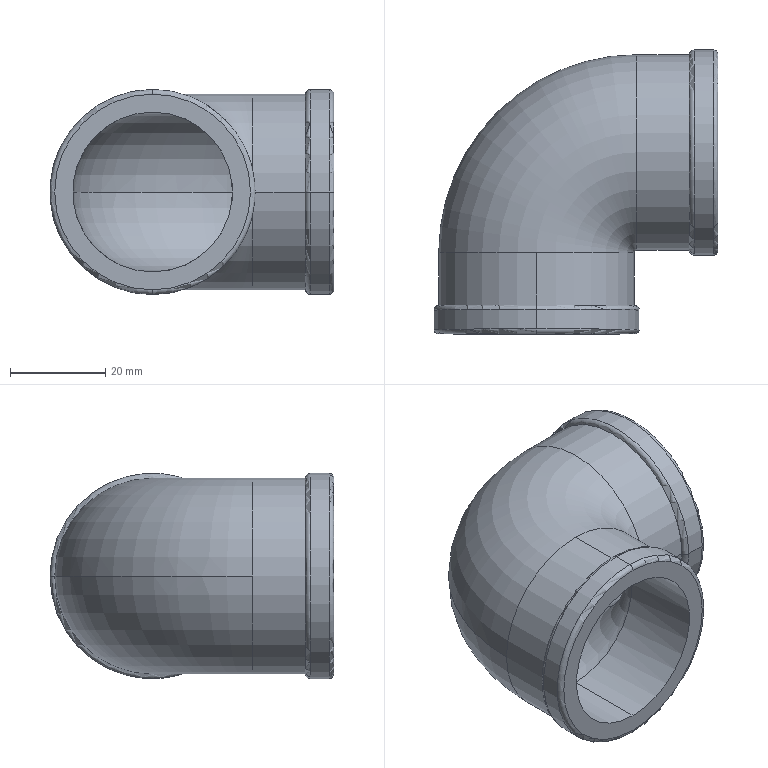Part | SolidWorks | features BossThin 2, Fillet 2, Sweep 1 | 1 solid | 26 faces | box 59.5 x 59.5 x 43 mm | volume 30865 mm3 | torus 12 | cylinder 12 | plane 2 | commonest cylinder face diameters 33.5 x4 41 x4 43 x4
STEP:
#1=CARTESIAN_POINT('',(-16.75,17.,0.));
#2=VERTEX_POINT('',#1);
#3=CARTESIAN_POINT('',(0.,17.,16.75));
#4=VERTEX_POINT('',#3);
#5=CARTESIAN_POINT('',(0.,17.,0.));
#6=DIRECTION('',(0.,1.,0.));
#7=DIRECTION('',(0.,0.,1.));
#8=AXIS2_PLACEMENT_3D('',#5,#6,#7);
#9=CIRCLE('',#8,16.75);
#10=EDGE_CURVE('',#2,#4,#9,.T.);
#11=ORIENTED_EDGE('',*,*,#10,.F.);
#12=CARTESIAN_POINT('',(21.,54.75,0.));
#13=VERTEX_POINT('',#12);
#14=CARTESIAN_POINT('',(21.,17.,0.));
#15=DIRECTION('',(0.,0.,-1.));
#16=DIRECTION('',(-1.,0.,0.));
#17=AXIS2_PLACEMENT_3D('',#14,#15,#16);
#18=CIRCLE('',#17,37.75);
#19=EDGE_CURVE('',#2,#13,#18,.T.);
#20=ORIENTED_EDGE('',*,*,#19,.T.);
#21=CARTESIAN_POINT('',(21.,21.25,0.));
#22=VERTEX_POINT('',#21);
#23=CARTESIAN_POINT('',(21.,38.,0.));
#24=DIRECTION('',(1.,0.,0.));
#25=DIRECTION('',(0.,0.,1.));
#26=AXIS2_PLACEMENT_3D('',#23,#24,#25);
#27=CIRCLE('',#26,16.75);
#28=EDGE_CURVE('',#13,#22,#27,.T.);
#29=ORIENTED_EDGE('',*,*,#28,.T.);
#30=CARTESIAN_POINT('',(16.75,17.,0.));
#31=VERTEX_POINT('',#30);
#32=CARTESIAN_POINT('',(21.,17.,0.));
#33=DIRECTION('',(0.,0.,-1.));
#34=DIRECTION('',(-1.,0.,0.));
#35=AXIS2_PLACEMENT_3D('',#32,#33,#34);
#36=CIRCLE('',#35,4.25);
#37=EDGE_CURVE('',#31,#22,#36,.T.);
#38=ORIENTED_EDGE('',*,*,#37,.F.);
#39=CARTESIAN_POINT('',(0.,17.,0.));
#40=DIRECTION('',(0.,1.,0.));
#41=DIRECTION('',(0.,0.,1.));
#42=AXIS2_PLACEMENT_3D('',#39,#40,#41);
#43=CIRCLE('',#42,16.75);
#44=EDGE_CURVE('',#4,#31,#43,.T.);
#45=ORIENTED_EDGE('',*,*,#44,.F.);
#46=EDGE_LOOP('',(#11,#20,#29,#38,#45));
#47=FACE_OUTER_BOUND('',#46,.T.);
#48=CARTESIAN_POINT('',(21.,17.,0.));
#49=DIRECTION('',(0.,0.,-1.));
#50=DIRECTION('',(-1.,0.,0.));
#51=AXIS2_PLACEMENT_3D('',#48,#49,#50);
#52=TOROIDAL_SURFACE('',#51,21.,16.75);
#53=ADVANCED_FACE('',(#47),#52,.F.);
#54=CARTESIAN_POINT('',(0.,17.,-20.5));
#55=VERTEX_POINT('',#54);
#56=CARTESIAN_POINT('',(-20.5,17.,0.));
#57=VERTEX_POINT('',#56);
#58=CARTESIAN_POINT('',(0.,17.,0.));
#59=DIRECTION('',(0.,1.,0.));
#60=DIRECTION('',(0.,0.,1.));
#61=AXIS2_PLACEMENT_3D('',#58,#59,#60);
#62=CIRCLE('',#61,20.5);
#63=EDGE_CURVE('',#55,#57,#62,.T.);
#64=ORIENTED_EDGE('',*,*,#63,.T.);
#65=CARTESIAN_POINT('',(21.,58.5,0.));
#66=VERTEX_POINT('',#65);
#67=CARTESIAN_POINT('',(21.,17.,0.));
#68=DIRECTION('',(0.,0.,-1.));
#69=DIRECTION('',(-1.,0.,0.));
#70=AXIS2_PLACEMENT_3D('',#67,#68,#69);
#71=CIRCLE('',#70,41.5);
#72=EDGE_CURVE('',#57,#66,#71,.T.);
#73=ORIENTED_EDGE('',*,*,#72,.T.);
#74=CARTESIAN_POINT('',(21.,17.5,0.));
#75=VERTEX_POINT('',#74);
#76=CARTESIAN_POINT('',(21.,38.,0.));
#77=DIRECTION('',(1.,0.,0.));
#78=DIRECTION('',(0.,0.,1.));
#79=AXIS2_PLACEMENT_3D('',#76,#77,#78);
#80=CIRCLE('',#79,20.5);
#81=EDGE_CURVE('',#75,#66,#80,.T.);
#82=ORIENTED_EDGE('',*,*,#81,.F.);
#83=CARTESIAN_POINT('',(20.5,17.,0.));
#84=VERTEX_POINT('',#83);
#85=CARTESIAN_POINT('',(21.,17.,0.));
#86=DIRECTION('',(0.,0.,-1.));
#87=DIRECTION('',(-1.,0.,0.));
#88=AXIS2_PLACEMENT_3D('',#85,#86,#87);
#89=CIRCLE('',#88,0.5);
#90=EDGE_CURVE('',#84,#75,#89,.T.);
#91=ORIENTED_EDGE('',*,*,#90,.F.);
#92=CARTESIAN_POINT('',(0.,17.,0.));
#93=DIRECTION('',(0.,1.,0.));
#94=DIRECTION('',(0.,0.,1.));
#95=AXIS2_PLACEMENT_3D('',#92,#93,#94);
#96=CIRCLE('',#95,20.5);
#97=EDGE_CURVE('',#84,#55,#96,.T.);
#98=ORIENTED_EDGE('',*,*,#97,.T.);
#99=EDGE_LOOP('',(#64,#73,#82,#91,#98));
#100=FACE_OUTER_BOUND('',#99,.T.);
#101=CARTESIAN_POINT('',(21.,17.,0.));
#102=DIRECTION('',(0.,0.,-1.));
#103=DIRECTION('',(-1.,0.,0.));
#104=AXIS2_PLACEMENT_3D('',#101,#102,#103);
#105=TOROIDAL_SURFACE('',#104,21.,20.5);
#106=ADVANCED_FACE('',(#100),#105,.T.);
#107=CARTESIAN_POINT('',(37.,16.5,0.));
#108=VERTEX_POINT('',#107);
#109=CARTESIAN_POINT('',(37.,59.5,0.));
#110=VERTEX_POINT('',#109);
#111=CARTESIAN_POINT('',(37.,38.,0.));
#112=DIRECTION('',(-1.,0.,0.));
#113=DIRECTION('',(0.,1.,0.));
#114=AXIS2_PLACEMENT_3D('',#111,#112,#113);
#115=CIRCLE('',#114,21.5);
#116=EDGE_CURVE('',#108,#110,#115,.T.);
#117=ORIENTED_EDGE('',*,*,#116,.F.);
#118=CARTESIAN_POINT('',(38.,17.5,0.));
#119=VERTEX_POINT('',#118);
#120=CARTESIAN_POINT('',(37.,17.5,0.));
#121=DIRECTION('',(0.,0.,1.));
#122=DIRECTION('',(0.,-1.,0.));
#123=AXIS2_PLACEMENT_3D('',#120,#121,#122);
#124=CIRCLE('',#123,1.);
#125=EDGE_CURVE('',#108,#119,#124,.T.);
#126=ORIENTED_EDGE('',*,*,#125,.T.);
#127=CARTESIAN_POINT('',(38.,58.5,0.));
#128=VERTEX_POINT('',#127);
#129=CARTESIAN_POINT('',(38.,38.,0.));
#130=DIRECTION('',(1.,0.,0.));
#131=DIRECTION('',(0.,1.,0.));
#132=AXIS2_PLACEMENT_3D('',#129,#130,#131);
#133=CIRCLE('',#132,20.5);
#134=EDGE_CURVE('',#128,#119,#133,.T.);
#135=ORIENTED_EDGE('',*,*,#134,.F.);
#136=CARTESIAN_POINT('',(37.,58.5,0.));
#137=DIRECTION('',(0.,0.,-1.));
#138=DIRECTION('',(-1.,0.,0.));
#139=AXIS2_PLACEMENT_3D('',#136,#137,#138);
#140=CIRCLE('',#139,1.);
#141=EDGE_CURVE('',#110,#128,#140,.T.);
#142=ORIENTED_EDGE('',*,*,#141,.F.);
#143=EDGE_LOOP('',(#117,#126,#135,#142));
#144=FACE_OUTER_BOUND('',#143,.T.);
#145=CARTESIAN_POINT('',(37.,38.,0.));
#146=DIRECTION('',(1.,0.,0.));
#147=DIRECTION('',(0.,1.,0.));
#148=AXIS2_PLACEMENT_3D('',#145,#146,#147);
#149=TOROIDAL_SURFACE('',#148,20.5,1.);
#150=ADVANCED_FACE('',(#144),#149,.T.);
#151=CARTESIAN_POINT('',(32.,58.5,0.));
#152=VERTEX_POINT('',#151);
#153=CARTESIAN_POINT('',(32.,17.5,0.));
#154=VERTEX_POINT('',#153);
#155=CARTESIAN_POINT('',(32.,38.,0.));
#156=DIRECTION('',(1.,0.,0.));
#157=DIRECTION('',(0.,1.,0.));
#158=AXIS2_PLACEMENT_3D('',#155,#156,#157);
#159=CIRCLE('',#158,20.5);
#160=EDGE_CURVE('',#152,#154,#159,.T.);
#161=ORIENTED_EDGE('',*,*,#160,.T.);
#162=CARTESIAN_POINT('',(33.,16.5,0.));
#163=VERTEX_POINT('',#162);
#164=CARTESIAN_POINT('',(33.,17.5,0.));
#165=DIRECTION('',(0.,0.,1.));
#166=DIRECTION('',(0.,-1.,0.));
#167=AXIS2_PLACEMENT_3D('',#164,#165,#166);
#168=CIRCLE('',#167,1.);
#169=EDGE_CURVE('',#154,#163,#168,.T.);
#170=ORIENTED_EDGE('',*,*,#169,.T.);
#171=CARTESIAN_POINT('',(33.,59.5,0.));
#172=VERTEX_POINT('',#171);
#173=CARTESIAN_POINT('',(33.,38.,0.));
#174=DIRECTION('',(1.,0.,0.));
#175=DIRECTION('',(0.,1.,0.));
#176=AXIS2_PLACEMENT_3D('',#173,#174,#175);
#177=CIRCLE('',#176,21.5);
#178=EDGE_CURVE('',#172,#163,#177,.T.);
#179=ORIENTED_EDGE('',*,*,#178,.F.);
#180=CARTESIAN_POINT('',(33.,58.5,0.));
#181=DIRECTION('',(0.,0.,-1.));
#182=DIRECTION('',(-1.,0.,0.));
#183=AXIS2_PLACEMENT_3D('',#180,#181,#182);
#184=CIRCLE('',#183,1.);
#185=EDGE_CURVE('',#152,#172,#184,.T.);
#186=ORIENTED_EDGE('',*,*,#185,.F.);
#187=EDGE_LOOP('',(#161,#170,#179,#186));
#188=FACE_OUTER_BOUND('',#187,.T.);
#189=CARTESIAN_POINT('',(33.,38.,0.));
#190=DIRECTION('',(1.,0.,0.));
#191=DIRECTION('',(0.,1.,0.));
#192=AXIS2_PLACEMENT_3D('',#189,#190,#191);
#193=TOROIDAL_SURFACE('',#192,20.5,1.);
#194=ADVANCED_FACE('',(#188),#193,.T.);
#195=ORIENTED_EDGE('',*,*,#178,.T.);
#196=CARTESIAN_POINT('',(32.,16.5,0.));
#197=DIRECTION('',(1.,0.,0.));
#198=VECTOR('',#197,1000.);
#199=LINE('',#196,#198);
#200=EDGE_CURVE('',#163,#108,#199,.T.);
#201=ORIENTED_EDGE('',*,*,#200,.T.);
#202=ORIENTED_EDGE('',*,*,#116,.T.);
#203=CARTESIAN_POINT('',(32.,59.5,0.));
#204=DIRECTION('',(1.,0.,0.));
#205=VECTOR('',#204,1000.);
#206=LINE('',#203,#205);
#207=EDGE_CURVE('',#172,#110,#206,.T.);
#208=ORIENTED_EDGE('',*,*,#207,.F.);
#209=EDGE_LOOP('',(#195,#201,#202,#208));
#210=FACE_OUTER_BOUND('',#209,.T.);
#211=CARTESIAN_POINT('',(32.,38.,0.));
#212=DIRECTION('',(1.,0.,0.));
#213=DIRECTION('',(0.,1.,0.));
#214=AXIS2_PLACEMENT_3D('',#211,#212,#213);
#215=CYLINDRICAL_SURFACE('',#214,21.5);
#216=ADVANCED_FACE('',(#210),#215,.T.);
#217=CARTESIAN_POINT('',(0.,0.,-20.5));
#218=VERTEX_POINT('',#217);
#219=CARTESIAN_POINT('',(0.,0.,20.5));
#220=VERTEX_POINT('',#219);
#221=CARTESIAN_POINT('',(0.,0.,0.));
#222=DIRECTION('',(0.,-1.,0.));
#223=DIRECTION('',(0.,0.,1.));
#224=AXIS2_PLACEMENT_3D('',#221,#222,#223);
#225=CIRCLE('',#224,20.5);
#226=EDGE_CURVE('',#218,#220,#225,.T.);
#227=ORIENTED_EDGE('',*,*,#226,.F.);
#228=CARTESIAN_POINT('',(0.,1.,-21.5));
#229=VERTEX_POINT('',#228);
#230=CARTESIAN_POINT('',(0.,1.,-20.5));
#231=DIRECTION('',(1.,0.,0.));
#232=DIRECTION('',(0.,0.,-1.));
#233=AXIS2_PLACEMENT_3D('',#230,#231,#232);
#234=CIRCLE('',#233,1.);
#235=EDGE_CURVE('',#218,#229,#234,.T.);
#236=ORIENTED_EDGE('',*,*,#235,.T.);
#237=CARTESIAN_POINT('',(0.,1.,21.5));
#238=VERTEX_POINT('',#237);
#239=CARTESIAN_POINT('',(0.,1.,0.));
#240=DIRECTION('',(0.,1.,0.));
#241=DIRECTION('',(0.,0.,1.));
#242=AXIS2_PLACEMENT_3D('',#239,#240,#241);
#243=CIRCLE('',#242,21.5);
#244=EDGE_CURVE('',#238,#229,#243,.T.);
#245=ORIENTED_EDGE('',*,*,#244,.F.);
#246=CARTESIAN_POINT('',(0.,1.,20.5));
#247=DIRECTION('',(-1.,0.,0.));
#248=DIRECTION('',(0.,0.,1.));
#249=AXIS2_PLACEMENT_3D('',#246,#247,#248);
#250=CIRCLE('',#249,1.);
#251=EDGE_CURVE('',#220,#238,#250,.T.);
#252=ORIENTED_EDGE('',*,*,#251,.F.);
#253=EDGE_LOOP('',(#227,#236,#245,#252));
#254=FACE_OUTER_BOUND('',#253,.T.);
#255=CARTESIAN_POINT('',(0.,1.,0.));
#256=DIRECTION('',(0.,1.,0.));
#257=DIRECTION('',(0.,0.,1.));
#258=AXIS2_PLACEMENT_3D('',#255,#256,#257);
#259=TOROIDAL_SURFACE('',#258,20.5,1.);
#260=ADVANCED_FACE('',(#254),#259,.T.);
#261=CARTESIAN_POINT('',(0.,6.,-20.5));
#262=VERTEX_POINT('',#261);
#263=CARTESIAN_POINT('',(0.,6.,20.5));
#264=VERTEX_POINT('',#263);
#265=CARTESIAN_POINT('',(0.,6.,0.));
#266=DIRECTION('',(0.,-1.,0.));
#267=DIRECTION('',(0.,0.,-1.));
#268=AXIS2_PLACEMENT_3D('',#265,#266,#267);
#269=CIRCLE('',#268,20.5);
#270=EDGE_CURVE('',#262,#264,#269,.T.);
#271=ORIENTED_EDGE('',*,*,#270,.T.);
#272=CARTESIAN_POINT('',(0.,5.,21.5));
#273=VERTEX_POINT('',#272);
#274=CARTESIAN_POINT('',(0.,5.,20.5));
#275=DIRECTION('',(1.,0.,0.));
#276=DIRECTION('',(0.,0.,-1.));
#277=AXIS2_PLACEMENT_3D('',#274,#275,#276);
#278=CIRCLE('',#277,1.);
#279=EDGE_CURVE('',#264,#273,#278,.T.);
#280=ORIENTED_EDGE('',*,*,#279,.T.);
#281=CARTESIAN_POINT('',(0.,5.,-21.5));
#282=VERTEX_POINT('',#281);
#283=CARTESIAN_POINT('',(0.,5.,0.));
#284=DIRECTION('',(0.,-1.,0.));
#285=DIRECTION('',(0.,0.,-1.));
#286=AXIS2_PLACEMENT_3D('',#283,#284,#285);
#287=CIRCLE('',#286,21.5);
#288=EDGE_CURVE('',#282,#273,#287,.T.);
#289=ORIENTED_EDGE('',*,*,#288,.F.);
#290=CARTESIAN_POINT('',(0.,5.,-20.5));
#291=DIRECTION('',(-1.,0.,0.));
#292=DIRECTION('',(0.,0.,1.));
#293=AXIS2_PLACEMENT_3D('',#290,#291,#292);
#294=CIRCLE('',#293,1.);
#295=EDGE_CURVE('',#262,#282,#294,.T.);
#296=ORIENTED_EDGE('',*,*,#295,.F.);
#297=EDGE_LOOP('',(#271,#280,#289,#296));
#298=FACE_OUTER_BOUND('',#297,.T.);
#299=CARTESIAN_POINT('',(0.,5.,0.));
#300=DIRECTION('',(0.,-1.,0.));
#301=DIRECTION('',(0.,0.,-1.));
#302=AXIS2_PLACEMENT_3D('',#299,#300,#301);
#303=TOROIDAL_SURFACE('',#302,20.5,1.);
#304=ADVANCED_FACE('',(#298),#303,.T.);
#305=ORIENTED_EDGE('',*,*,#288,.T.);
#306=CARTESIAN_POINT('',(0.,6.,21.5));
#307=DIRECTION('',(0.,-1.,0.));
#308=VECTOR('',#307,1000.);
#309=LINE('',#306,#308);
#310=EDGE_CURVE('',#273,#238,#309,.T.);
#311=ORIENTED_EDGE('',*,*,#310,.T.);
#312=ORIENTED_EDGE('',*,*,#244,.T.);
#313=CARTESIAN_POINT('',(0.,6.,-21.5));
#314=DIRECTION('',(0.,-1.,0.));
#315=VECTOR('',#314,1000.);
#316=LINE('',#313,#315);
#317=EDGE_CURVE('',#282,#229,#316,.T.);
#318=ORIENTED_EDGE('',*,*,#317,.F.);
#319=EDGE_LOOP('',(#305,#311,#312,#318));
#320=FACE_OUTER_BOUND('',#319,.T.);
#321=CARTESIAN_POINT('',(0.,6.,0.));
#322=DIRECTION('',(0.,-1.,0.));
#323=DIRECTION('',(0.,0.,-1.));
#324=AXIS2_PLACEMENT_3D('',#321,#322,#323);
#325=CYLINDRICAL_SURFACE('',#324,21.5);
#326=ADVANCED_FACE('',(#320),#325,.T.);
#327=CARTESIAN_POINT('',(0.,17.,-16.75));
#328=VERTEX_POINT('',#327);
#329=CARTESIAN_POINT('',(0.,17.,0.));
#330=DIRECTION('',(0.,1.,0.));
#331=DIRECTION('',(0.,0.,1.));
#332=AXIS2_PLACEMENT_3D('',#329,#330,#331);
#333=CIRCLE('',#332,16.75);
#334=EDGE_CURVE('',#328,#2,#333,.T.);
#335=ORIENTED_EDGE('',*,*,#334,.T.);
#336=ORIENTED_EDGE('',*,*,#10,.T.);
#337=CARTESIAN_POINT('',(0.,0.,16.75));
#338=VERTEX_POINT('',#337);
#339=CARTESIAN_POINT('',(0.,17.,16.75));
#340=DIRECTION('',(0.,-1.,0.));
#341=VECTOR('',#340,1000.);
#342=LINE('',#339,#341);
#343=EDGE_CURVE('',#4,#338,#342,.T.);
#344=ORIENTED_EDGE('',*,*,#343,.T.);
#345=CARTESIAN_POINT('',(0.,0.,-16.75));
#346=VERTEX_POINT('',#345);
#347=CARTESIAN_POINT('',(0.,0.,0.));
#348=DIRECTION('',(0.,1.,0.));
#349=DIRECTION('',(0.,0.,1.));
#350=AXIS2_PLACEMENT_3D('',#347,#348,#349);
#351=CIRCLE('',#350,16.75);
#352=EDGE_CURVE('',#346,#338,#351,.T.);
#353=ORIENTED_EDGE('',*,*,#352,.F.);
#354=CARTESIAN_POINT('',(0.,17.,-16.75));
#355=DIRECTION('',(0.,-1.,0.));
#356=VECTOR('',#355,1000.);
#357=LINE('',#354,#356);
#358=EDGE_CURVE('',#328,#346,#357,.T.);
#359=ORIENTED_EDGE('',*,*,#358,.F.);
#360=EDGE_LOOP('',(#335,#336,#344,#353,#359));
#361=FACE_OUTER_BOUND('',#360,.T.);
#362=CARTESIAN_POINT('',(0.,17.,0.));
#363=DIRECTION('',(0.,-1.,0.));
#364=DIRECTION('',(0.,0.,-1.));
#365=AXIS2_PLACEMENT_3D('',#362,#363,#364);
#366=CYLINDRICAL_SURFACE('',#365,16.75);
#367=ADVANCED_FACE('',(#361),#366,.F.);
#368=CARTESIAN_POINT('',(21.,38.,0.));
#369=DIRECTION('',(1.,0.,0.));
#370=DIRECTION('',(0.,0.,1.));
#371=AXIS2_PLACEMENT_3D('',#368,#369,#370);
#372=CIRCLE('',#371,16.75);
#373=EDGE_CURVE('',#22,#13,#372,.T.);
#374=ORIENTED_EDGE('',*,*,#373,.F.);
#375=CARTESIAN_POINT('',(38.,21.25,0.));
#376=VERTEX_POINT('',#375);
#377=CARTESIAN_POINT('',(21.,21.25,0.));
#378=DIRECTION('',(1.,0.,0.));
#379=VECTOR('',#378,1000.);
#380=LINE('',#377,#379);
#381=EDGE_CURVE('',#22,#376,#380,.T.);
#382=ORIENTED_EDGE('',*,*,#381,.T.);
#383=CARTESIAN_POINT('',(38.,54.75,0.));
#384=VERTEX_POINT('',#383);
#385=CARTESIAN_POINT('',(38.,38.,0.));
#386=DIRECTION('',(1.,0.,0.));
#387=DIRECTION('',(0.,0.,1.));
#388=AXIS2_PLACEMENT_3D('',#385,#386,#387);
#389=CIRCLE('',#388,16.75);
#390=EDGE_CURVE('',#376,#384,#389,.T.);
#391=ORIENTED_EDGE('',*,*,#390,.T.);
#392=CARTESIAN_POINT('',(21.,54.75,0.));
#393=DIRECTION('',(1.,0.,0.));
#394=VECTOR('',#393,1000.);
#395=LINE('',#392,#394);
#396=EDGE_CURVE('',#13,#384,#395,.T.);
#397=ORIENTED_EDGE('',*,*,#396,.F.);
#398=EDGE_LOOP('',(#374,#382,#391,#397));
#399=FACE_OUTER_BOUND('',#398,.T.);
#400=CARTESIAN_POINT('',(21.,38.,0.));
#401=DIRECTION('',(1.,0.,0.));
#402=DIRECTION('',(0.,1.,0.));
#403=AXIS2_PLACEMENT_3D('',#400,#401,#402);
#404=CYLINDRICAL_SURFACE('',#403,16.75);
#405=ADVANCED_FACE('',(#399),#404,.F.);
#406=CARTESIAN_POINT('',(0.,17.,20.5));
#407=VERTEX_POINT('',#406);
#408=CARTESIAN_POINT('',(0.,17.,0.));
#409=DIRECTION('',(0.,1.,0.));
#410=DIRECTION('',(0.,0.,1.));
#411=AXIS2_PLACEMENT_3D('',#408,#409,#410);
#412=CIRCLE('',#411,20.5);
#413=EDGE_CURVE('',#407,#84,#412,.T.);
#414=ORIENTED_EDGE('',*,*,#413,.F.);
#415=CARTESIAN_POINT('',(0.,17.,20.5));
#416=DIRECTION('',(0.,-1.,0.));
#417=VECTOR('',#416,1000.);
#418=LINE('',#415,#417);
#419=EDGE_CURVE('',#407,#264,#418,.T.);
#420=ORIENTED_EDGE('',*,*,#419,.T.);
#421=ORIENTED_EDGE('',*,*,#270,.F.);
#422=CARTESIAN_POINT('',(0.,17.,-20.5));
#423=DIRECTION('',(0.,-1.,0.));
#424=VECTOR('',#423,1000.);
#425=LINE('',#422,#424);
#426=EDGE_CURVE('',#55,#262,#425,.T.);
#427=ORIENTED_EDGE('',*,*,#426,.F.);
#428=ORIENTED_EDGE('',*,*,#97,.F.);
#429=EDGE_LOOP('',(#414,#420,#421,#427,#428));
#430=FACE_OUTER_BOUND('',#429,.T.);
#431=CARTESIAN_POINT('',(0.,17.,0.));
#432=DIRECTION('',(0.,-1.,0.));
#433=DIRECTION('',(0.,0.,-1.));
#434=AXIS2_PLACEMENT_3D('',#431,#432,#433);
#435=CYLINDRICAL_SURFACE('',#434,20.5);
#436=ADVANCED_FACE('',(#430),#435,.T.);
#437=CARTESIAN_POINT('',(21.,38.,0.));
#438=DIRECTION('',(1.,0.,0.));
#439=DIRECTION('',(0.,0.,1.));
#440=AXIS2_PLACEMENT_3D('',#437,#438,#439);
#441=CIRCLE('',#440,20.5);
#442=EDGE_CURVE('',#66,#75,#441,.T.);
#443=ORIENTED_EDGE('',*,*,#442,.T.);
#444=CARTESIAN_POINT('',(21.,17.5,0.));
#445=DIRECTION('',(1.,0.,0.));
#446=VECTOR('',#445,1000.);
#447=LINE('',#444,#446);
#448=EDGE_CURVE('',#75,#154,#447,.T.);
#449=ORIENTED_EDGE('',*,*,#448,.T.);
#450=ORIENTED_EDGE('',*,*,#160,.F.);
#451=CARTESIAN_POINT('',(21.,58.5,0.));
#452=DIRECTION('',(1.,0.,0.));
#453=VECTOR('',#452,1000.);
#454=LINE('',#451,#453);
#455=EDGE_CURVE('',#66,#152,#454,.T.);
#456=ORIENTED_EDGE('',*,*,#455,.F.);
#457=EDGE_LOOP('',(#443,#449,#450,#456));
#458=FACE_OUTER_BOUND('',#457,.T.);
#459=CARTESIAN_POINT('',(21.,38.,0.));
#460=DIRECTION('',(1.,0.,0.));
#461=DIRECTION('',(0.,1.,0.));
#462=AXIS2_PLACEMENT_3D('',#459,#460,#461);
#463=CYLINDRICAL_SURFACE('',#462,20.5);
#464=ADVANCED_FACE('',(#458),#463,.T.);
#465=ORIENTED_EDGE('',*,*,#448,.F.);
#466=ORIENTED_EDGE('',*,*,#81,.T.);
#467=ORIENTED_EDGE('',*,*,#455,.T.);
#468=CARTESIAN_POINT('',(32.,38.,0.));
#469=DIRECTION('',(1.,0.,0.));
#470=DIRECTION('',(0.,1.,0.));
#471=AXIS2_PLACEMENT_3D('',#468,#469,#470);
#472=CIRCLE('',#471,20.5);
#473=EDGE_CURVE('',#154,#152,#472,.T.);
#474=ORIENTED_EDGE('',*,*,#473,.F.);
#475=EDGE_LOOP('',(#465,#466,#467,#474));
#476=FACE_OUTER_BOUND('',#475,.T.);
#477=CARTESIAN_POINT('',(21.,38.,0.));
#478=DIRECTION('',(1.,0.,0.));
#479=DIRECTION('',(0.,1.,0.));
#480=AXIS2_PLACEMENT_3D('',#477,#478,#479);
#481=CYLINDRICAL_SURFACE('',#480,20.5);
#482=ADVANCED_FACE('',(#476),#481,.T.);
#483=ORIENTED_EDGE('',*,*,#419,.F.);
#484=CARTESIAN_POINT('',(0.,17.,0.));
#485=DIRECTION('',(0.,1.,0.));
#486=DIRECTION('',(0.,0.,1.));
#487=AXIS2_PLACEMENT_3D('',#484,#485,#486);
#488=CIRCLE('',#487,20.5);
#489=EDGE_CURVE('',#57,#407,#488,.T.);
#490=ORIENTED_EDGE('',*,*,#489,.F.);
#491=ORIENTED_EDGE('',*,*,#63,.F.);
#492=ORIENTED_EDGE('',*,*,#426,.T.);
#493=CARTESIAN_POINT('',(0.,6.,0.));
#494=DIRECTION('',(0.,-1.,0.));
#495=DIRECTION('',(0.,0.,-1.));
#496=AXIS2_PLACEMENT_3D('',#493,#494,#495);
#497=CIRCLE('',#496,20.5);
#498=EDGE_CURVE('',#264,#262,#497,.T.);
#499=ORIENTED_EDGE('',*,*,#498,.F.);
#500=EDGE_LOOP('',(#483,#490,#491,#492,#499));
#501=FACE_OUTER_BOUND('',#500,.T.);
#502=CARTESIAN_POINT('',(0.,17.,0.));
#503=DIRECTION('',(0.,-1.,0.));
#504=DIRECTION('',(0.,0.,-1.));
#505=AXIS2_PLACEMENT_3D('',#502,#503,#504);
#506=CYLINDRICAL_SURFACE('',#505,20.5);
#507=ADVANCED_FACE('',(#501),#506,.T.);
#508=ORIENTED_EDGE('',*,*,#381,.F.);
#509=ORIENTED_EDGE('',*,*,#28,.F.);
#510=ORIENTED_EDGE('',*,*,#396,.T.);
#511=CARTESIAN_POINT('',(38.,38.,0.));
#512=DIRECTION('',(1.,0.,0.));
#513=DIRECTION('',(0.,0.,1.));
#514=AXIS2_PLACEMENT_3D('',#511,#512,#513);
#515=CIRCLE('',#514,16.75);
#516=EDGE_CURVE('',#384,#376,#515,.T.);
#517=ORIENTED_EDGE('',*,*,#516,.T.);
#518=EDGE_LOOP('',(#508,#509,#510,#517));
#519=FACE_OUTER_BOUND('',#518,.T.);
#520=CARTESIAN_POINT('',(21.,38.,0.));
#521=DIRECTION('',(1.,0.,0.));
#522=DIRECTION('',(0.,1.,0.));
#523=AXIS2_PLACEMENT_3D('',#520,#521,#522);
#524=CYLINDRICAL_SURFACE('',#523,16.75);
#525=ADVANCED_FACE('',(#519),#524,.F.);
#526=ORIENTED_EDGE('',*,*,#72,.F.);
#527=ORIENTED_EDGE('',*,*,#489,.T.);
#528=ORIENTED_EDGE('',*,*,#413,.T.);
#529=ORIENTED_EDGE('',*,*,#90,.T.);
#530=ORIENTED_EDGE('',*,*,#442,.F.);
#531=EDGE_LOOP('',(#526,#527,#528,#529,#530));
#532=FACE_OUTER_BOUND('',#531,.T.);
#533=CARTESIAN_POINT('',(21.,17.,0.));
#534=DIRECTION('',(0.,0.,-1.));
#535=DIRECTION('',(-1.,0.,0.));
#536=AXIS2_PLACEMENT_3D('',#533,#534,#535);
#537=TOROIDAL_SURFACE('',#536,21.,20.5);
#538=ADVANCED_FACE('',(#532),#537,.T.);
#539=ORIENTED_EDGE('',*,*,#19,.F.);
#540=ORIENTED_EDGE('',*,*,#334,.F.);
#541=CARTESIAN_POINT('',(0.,17.,0.));
#542=DIRECTION('',(0.,1.,0.));
#543=DIRECTION('',(0.,0.,1.));
#544=AXIS2_PLACEMENT_3D('',#541,#542,#543);
#545=CIRCLE('',#544,16.75);
#546=EDGE_CURVE('',#31,#328,#545,.T.);
#547=ORIENTED_EDGE('',*,*,#546,.F.);
#548=ORIENTED_EDGE('',*,*,#37,.T.);
#549=ORIENTED_EDGE('',*,*,#373,.T.);
#550=EDGE_LOOP('',(#539,#540,#547,#548,#549));
#551=FACE_OUTER_BOUND('',#550,.T.);
#552=CARTESIAN_POINT('',(21.,17.,0.));
#553=DIRECTION('',(0.,0.,-1.));
#554=DIRECTION('',(-1.,0.,0.));
#555=AXIS2_PLACEMENT_3D('',#552,#553,#554);
#556=TOROIDAL_SURFACE('',#555,21.,16.75);
#557=ADVANCED_FACE('',(#551),#556,.F.);
#558=ORIENTED_EDGE('',*,*,#343,.F.);
#559=ORIENTED_EDGE('',*,*,#44,.T.);
#560=ORIENTED_EDGE('',*,*,#546,.T.);
#561=ORIENTED_EDGE('',*,*,#358,.T.);
#562=CARTESIAN_POINT('',(0.,0.,0.));
#563=DIRECTION('',(0.,1.,0.));
#564=DIRECTION('',(0.,0.,1.));
#565=AXIS2_PLACEMENT_3D('',#562,#563,#564);
#566=CIRCLE('',#565,16.75);
#567=EDGE_CURVE('',#338,#346,#566,.T.);
#568=ORIENTED_EDGE('',*,*,#567,.F.);
#569=EDGE_LOOP('',(#558,#559,#560,#561,#568));
#570=FACE_OUTER_BOUND('',#569,.T.);
#571=CARTESIAN_POINT('',(0.,17.,0.));
#572=DIRECTION('',(0.,-1.,0.));
#573=DIRECTION('',(0.,0.,-1.));
#574=AXIS2_PLACEMENT_3D('',#571,#572,#573);
#575=CYLINDRICAL_SURFACE('',#574,16.75);
#576=ADVANCED_FACE('',(#570),#575,.F.);
#577=ORIENTED_EDGE('',*,*,#134,.T.);
#578=CARTESIAN_POINT('',(38.,38.,0.));
#579=DIRECTION('',(1.,0.,0.));
#580=DIRECTION('',(0.,1.,0.));
#581=AXIS2_PLACEMENT_3D('',#578,#579,#580);
#582=CIRCLE('',#581,20.5);
#583=EDGE_CURVE('',#119,#128,#582,.T.);
#584=ORIENTED_EDGE('',*,*,#583,.T.);
#585=EDGE_LOOP('',(#577,#584));
#586=FACE_OUTER_BOUND('',#585,.T.);
#587=ORIENTED_EDGE('',*,*,#516,.F.);
#588=ORIENTED_EDGE('',*,*,#390,.F.);
#589=EDGE_LOOP('',(#587,#588));
#590=FACE_BOUND('',#589,.T.);
#591=CARTESIAN_POINT('',(38.,38.,0.));
#592=DIRECTION('',(1.,0.,0.));
#593=DIRECTION('',(0.,0.,1.));
#594=AXIS2_PLACEMENT_3D('',#591,#592,#593);
#595=PLANE('',#594);
#596=ADVANCED_FACE('',(#586,#590),#595,.T.);
#597=CARTESIAN_POINT('',(0.,0.,0.));
#598=DIRECTION('',(0.,-1.,0.));
#599=DIRECTION('',(0.,0.,1.));
#600=AXIS2_PLACEMENT_3D('',#597,#598,#599);
#601=CIRCLE('',#600,20.5);
#602=EDGE_CURVE('',#220,#218,#601,.T.);
#603=ORIENTED_EDGE('',*,*,#602,.T.);
#604=ORIENTED_EDGE('',*,*,#226,.T.);
#605=EDGE_LOOP('',(#603,#604));
#606=FACE_OUTER_BOUND('',#605,.T.);
#607=ORIENTED_EDGE('',*,*,#352,.T.);
#608=ORIENTED_EDGE('',*,*,#567,.T.);
#609=EDGE_LOOP('',(#607,#608));
#610=FACE_BOUND('',#609,.T.);
#611=CARTESIAN_POINT('',(0.,0.,0.));
#612=DIRECTION('',(0.,1.,0.));
#613=DIRECTION('',(0.,0.,1.));
#614=AXIS2_PLACEMENT_3D('',#611,#612,#613);
#615=PLANE('',#614);
#616=ADVANCED_FACE('',(#606,#610),#615,.F.);
#617=ORIENTED_EDGE('',*,*,#310,.F.);
#618=CARTESIAN_POINT('',(0.,5.,0.));
#619=DIRECTION('',(0.,-1.,0.));
#620=DIRECTION('',(0.,0.,-1.));
#621=AXIS2_PLACEMENT_3D('',#618,#619,#620);
#622=CIRCLE('',#621,21.5);
#623=EDGE_CURVE('',#273,#282,#622,.T.);
#624=ORIENTED_EDGE('',*,*,#623,.T.);
#625=ORIENTED_EDGE('',*,*,#317,.T.);
#626=CARTESIAN_POINT('',(0.,1.,0.));
#627=DIRECTION('',(0.,1.,0.));
#628=DIRECTION('',(0.,0.,1.));
#629=AXIS2_PLACEMENT_3D('',#626,#627,#628);
#630=CIRCLE('',#629,21.5);
#631=EDGE_CURVE('',#229,#238,#630,.T.);
#632=ORIENTED_EDGE('',*,*,#631,.T.);
#633=EDGE_LOOP('',(#617,#624,#625,#632));
#634=FACE_OUTER_BOUND('',#633,.T.);
#635=CARTESIAN_POINT('',(0.,6.,0.));
#636=DIRECTION('',(0.,-1.,0.));
#637=DIRECTION('',(0.,0.,-1.));
#638=AXIS2_PLACEMENT_3D('',#635,#636,#637);
#639=CYLINDRICAL_SURFACE('',#638,21.5);
#640=ADVANCED_FACE('',(#634),#639,.T.);
#641=ORIENTED_EDGE('',*,*,#279,.F.);
#642=ORIENTED_EDGE('',*,*,#498,.T.);
#643=ORIENTED_EDGE('',*,*,#295,.T.);
#644=ORIENTED_EDGE('',*,*,#623,.F.);
#645=EDGE_LOOP('',(#641,#642,#643,#644));
#646=FACE_OUTER_BOUND('',#645,.T.);
#647=CARTESIAN_POINT('',(0.,5.,0.));
#648=DIRECTION('',(0.,-1.,0.));
#649=DIRECTION('',(0.,0.,-1.));
#650=AXIS2_PLACEMENT_3D('',#647,#648,#649);
#651=TOROIDAL_SURFACE('',#650,20.5,1.);
#652=ADVANCED_FACE('',(#646),#651,.T.);
#653=ORIENTED_EDGE('',*,*,#235,.F.);
#654=ORIENTED_EDGE('',*,*,#602,.F.);
#655=ORIENTED_EDGE('',*,*,#251,.T.);
#656=ORIENTED_EDGE('',*,*,#631,.F.);
#657=EDGE_LOOP('',(#653,#654,#655,#656));
#658=FACE_OUTER_BOUND('',#657,.T.);
#659=CARTESIAN_POINT('',(0.,1.,0.));
#660=DIRECTION('',(0.,1.,0.));
#661=DIRECTION('',(0.,0.,1.));
#662=AXIS2_PLACEMENT_3D('',#659,#660,#661);
#663=TOROIDAL_SURFACE('',#662,20.5,1.);
#664=ADVANCED_FACE('',(#658),#663,.T.);
#665=ORIENTED_EDGE('',*,*,#200,.F.);
#666=CARTESIAN_POINT('',(33.,38.,0.));
#667=DIRECTION('',(1.,0.,0.));
#668=DIRECTION('',(0.,1.,0.));
#669=AXIS2_PLACEMENT_3D('',#666,#667,#668);
#670=CIRCLE('',#669,21.5);
#671=EDGE_CURVE('',#163,#172,#670,.T.);
#672=ORIENTED_EDGE('',*,*,#671,.T.);
#673=ORIENTED_EDGE('',*,*,#207,.T.);
#674=CARTESIAN_POINT('',(37.,38.,0.));
#675=DIRECTION('',(-1.,0.,0.));
#676=DIRECTION('',(0.,1.,0.));
#677=AXIS2_PLACEMENT_3D('',#674,#675,#676);
#678=CIRCLE('',#677,21.5);
#679=EDGE_CURVE('',#110,#108,#678,.T.);
#680=ORIENTED_EDGE('',*,*,#679,.T.);
#681=EDGE_LOOP('',(#665,#672,#673,#680));
#682=FACE_OUTER_BOUND('',#681,.T.);
#683=CARTESIAN_POINT('',(32.,38.,0.));
#684=DIRECTION('',(1.,0.,0.));
#685=DIRECTION('',(0.,1.,0.));
#686=AXIS2_PLACEMENT_3D('',#683,#684,#685);
#687=CYLINDRICAL_SURFACE('',#686,21.5);
#688=ADVANCED_FACE('',(#682),#687,.T.);
#689=ORIENTED_EDGE('',*,*,#169,.F.);
#690=ORIENTED_EDGE('',*,*,#473,.T.);
#691=ORIENTED_EDGE('',*,*,#185,.T.);
#692=ORIENTED_EDGE('',*,*,#671,.F.);
#693=EDGE_LOOP('',(#689,#690,#691,#692));
#694=FACE_OUTER_BOUND('',#693,.T.);
#695=CARTESIAN_POINT('',(33.,38.,0.));
#696=DIRECTION('',(1.,0.,0.));
#697=DIRECTION('',(0.,1.,0.));
#698=AXIS2_PLACEMENT_3D('',#695,#696,#697);
#699=TOROIDAL_SURFACE('',#698,20.5,1.);
#700=ADVANCED_FACE('',(#694),#699,.T.);
#701=ORIENTED_EDGE('',*,*,#125,.F.);
#702=ORIENTED_EDGE('',*,*,#679,.F.);
#703=ORIENTED_EDGE('',*,*,#141,.T.);
#704=ORIENTED_EDGE('',*,*,#583,.F.);
#705=EDGE_LOOP('',(#701,#702,#703,#704));
#706=FACE_OUTER_BOUND('',#705,.T.);
#707=CARTESIAN_POINT('',(37.,38.,0.));
#708=DIRECTION('',(1.,0.,0.));
#709=DIRECTION('',(0.,1.,0.));
#710=AXIS2_PLACEMENT_3D('',#707,#708,#709);
#711=TOROIDAL_SURFACE('',#710,20.5,1.);
#712=ADVANCED_FACE('',(#706),#711,.T.);
#713=CLOSED_SHELL('',(#53,#106,#150,#194,#216,#260,#304,#326,#367,#405,#436,#464,#482,#507,#525,#538,#557,#576,#596,#616,#640,#652,#664,#688,#700,#712));
#714=MANIFOLD_SOLID_BREP('',#713);
#715=CARTESIAN_POINT('',(0.,0.,0.));
#716=DIRECTION('',(0.,0.,1.));
#717=DIRECTION('',(1.,0.,0.));
#718=AXIS2_PLACEMENT_3D('',#715,#716,#717);
#719=(LENGTH_UNIT()NAMED_UNIT(*)SI_UNIT(.MILLI.,.METRE.));
#720=UNCERTAINTY_MEASURE_WITH_UNIT(LENGTH_MEASURE(0.00001),#719,'','');
#721=(NAMED_UNIT(*)PLANE_ANGLE_UNIT()SI_UNIT($,.RADIAN.));
#722=(NAMED_UNIT(*)SI_UNIT($,.STERADIAN.)SOLID_ANGLE_UNIT());
#723=(GEOMETRIC_REPRESENTATION_CONTEXT(3)GLOBAL_UNCERTAINTY_ASSIGNED_CONTEXT((#720))GLOBAL_UNIT_ASSIGNED_CONTEXT((#719,#721,#722))REPRESENTATION_CONTEXT('',''));
#724=ADVANCED_BREP_SHAPE_REPRESENTATION('',(#714,#718),#723);